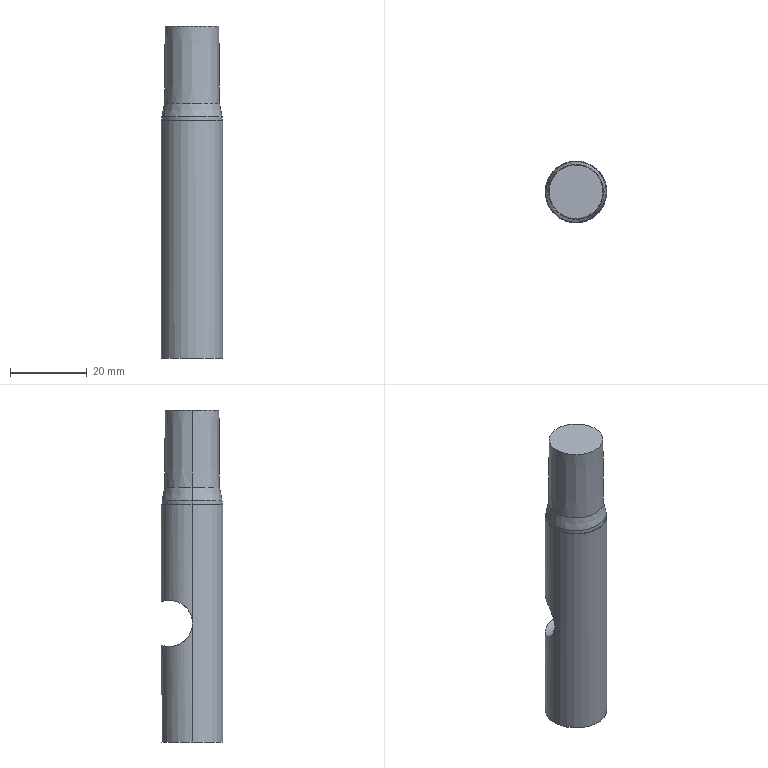Part | Creo | 1 solid | 13 faces | box 16.002 x 16 x 86.407 mm | volume 15399 mm3 | cylinder 6 | cone 4 | plane 3 | commonest cylinder face diameters 16 x3 15.678 x2 12 x1
STEP:
#1=CARTESIAN_POINT('',(0.,0.,0.));
#2=DIRECTION('',(0.,0.,1.));
#3=DIRECTION('',(1.,0.,0.));
#4=AXIS2_PLACEMENT_3D('',#1,#2,#3);
#5=CARTESIAN_POINT('',(104.477,27.678,-128.581));
#6=VERTEX_POINT('',#5);
#7=CARTESIAN_POINT('',(107.088,21.765,-123.596));
#8=VERTEX_POINT('',#7);
#9=CARTESIAN_POINT('',(104.477,27.678,-128.581));
#10=CARTESIAN_POINT('',(104.749,27.431,-128.581));
#11=CARTESIAN_POINT('',(105.24,26.915,-128.55));
#12=CARTESIAN_POINT('',(105.829,26.11,-128.393));
#13=CARTESIAN_POINT('',(106.284,25.299,-128.112));
#14=CARTESIAN_POINT('',(106.617,24.511,-127.704));
#15=CARTESIAN_POINT('',(106.849,23.756,-127.155));
#16=CARTESIAN_POINT('',(106.993,23.055,-126.45));
#17=CARTESIAN_POINT('',(107.064,22.455,-125.596));
#18=CARTESIAN_POINT('',(107.087,22.006,-124.63));
#19=CARTESIAN_POINT('',(107.088,21.826,-123.949));
#20=CARTESIAN_POINT('',(107.088,21.765,-123.596));
#21=B_SPLINE_CURVE_WITH_KNOTS('',3,(#9,#10,#11,#12,#13,#14,#15,#16,#17,#18,#19,#20),.UNSPECIFIED.,.F.,.F.,(4,1,1,1,1,1,1,1,1,4),(0.,0.1111,0.2222,0.3333,0.4444,0.5556,0.6667,0.7778,0.8889,1.),.UNSPECIFIED.);
#22=EDGE_CURVE('',#6,#8,#21,.T.);
#23=ORIENTED_EDGE('',*,*,#22,.T.);
#24=CARTESIAN_POINT('',(107.088,21.765,-121.572));
#25=VERTEX_POINT('',#24);
#26=CARTESIAN_POINT('',(107.088,21.765,-123.596));
#27=CARTESIAN_POINT('',(107.088,21.707,-123.258));
#28=CARTESIAN_POINT('',(107.087,21.65,-122.584));
#29=CARTESIAN_POINT('',(107.088,21.707,-121.909));
#30=CARTESIAN_POINT('',(107.088,21.765,-121.572));
#31=B_SPLINE_CURVE_WITH_KNOTS('',3,(#26,#27,#28,#29,#30),.UNSPECIFIED.,.F.,.F.,(4,1,4),(0.,0.5,1.),.UNSPECIFIED.);
#32=EDGE_CURVE('',#8,#25,#31,.T.);
#33=ORIENTED_EDGE('',*,*,#32,.T.);
#34=CARTESIAN_POINT('',(104.477,27.678,-116.581));
#35=VERTEX_POINT('',#34);
#36=CARTESIAN_POINT('',(107.088,21.765,-121.572));
#37=CARTESIAN_POINT('',(107.088,21.801,-121.361));
#38=CARTESIAN_POINT('',(107.087,21.894,-120.947));
#39=CARTESIAN_POINT('',(107.083,22.087,-120.374));
#40=CARTESIAN_POINT('',(107.067,22.369,-119.762));
#41=CARTESIAN_POINT('',(107.038,22.685,-119.235));
#42=CARTESIAN_POINT('',(106.982,23.089,-118.697));
#43=CARTESIAN_POINT('',(106.899,23.513,-118.25));
#44=CARTESIAN_POINT('',(106.79,23.947,-117.871));
#45=CARTESIAN_POINT('',(106.648,24.399,-117.547));
#46=CARTESIAN_POINT('',(106.469,24.864,-117.273));
#47=CARTESIAN_POINT('',(106.256,25.332,-117.051));
#48=CARTESIAN_POINT('',(105.99,25.823,-116.868));
#49=CARTESIAN_POINT('',(105.712,26.262,-116.745));
#50=CARTESIAN_POINT('',(105.379,26.72,-116.652));
#51=CARTESIAN_POINT('',(104.979,27.192,-116.595));
#52=CARTESIAN_POINT('',(104.654,27.517,-116.581));
#53=CARTESIAN_POINT('',(104.477,27.678,-116.581));
#54=B_SPLINE_CURVE_WITH_KNOTS('',3,(#36,#37,#38,#39,#40,#41,#42,#43,#44,#45,#46,#47,#48,#49,#50,#51,#52,#53),.UNSPECIFIED.,.F.,.F.,(4,1,1,1,1,1,1,1,1,1,1,1,1,1,1,4),(0.,0.06667,0.1333,0.2,0.2667,0.3333,0.4,0.4667,0.5333,0.6,0.6667,0.7333,0.8,0.8667,0.9333,1.),.UNSPECIFIED.);
#55=EDGE_CURVE('',#25,#35,#54,.T.);
#56=ORIENTED_EDGE('',*,*,#55,.T.);
#57=CARTESIAN_POINT('',(93.699,27.678,-116.581));
#58=VERTEX_POINT('',#57);
#59=CARTESIAN_POINT('',(104.158,27.97,-116.581));
#60=CARTESIAN_POINT('',(103.468,28.503,-116.623));
#61=CARTESIAN_POINT('',(102.306,29.13,-116.751));
#62=CARTESIAN_POINT('',(101.047,29.561,-116.881));
#63=CARTESIAN_POINT('',(99.717,29.78,-116.96));
#64=CARTESIAN_POINT('',(98.353,29.771,-116.957));
#65=CARTESIAN_POINT('',(97.016,29.532,-116.871));
#66=CARTESIAN_POINT('',(95.765,29.082,-116.739));
#67=CARTESIAN_POINT('',(94.636,28.453,-116.617));
#68=CARTESIAN_POINT('',(93.993,27.947,-116.581));
#69=CARTESIAN_POINT('',(93.699,27.678,-116.581));
#70=B_SPLINE_CURVE_WITH_KNOTS('',3,(#34,#59,#60,#61,#62,#63,#64,#65,#66,#67,#68,#69),.UNSPECIFIED.,.F.,.F.,(4,1,1,1,1,1,1,1,1,4),(0.,0.1111,0.2222,0.3333,0.4444,0.5556,0.6667,0.7778,0.8889,1.),.UNSPECIFIED.);
#71=EDGE_CURVE('',#35,#58,#70,.T.);
#72=ORIENTED_EDGE('',*,*,#71,.T.);
#73=CARTESIAN_POINT('',(91.087,21.766,-121.566));
#74=VERTEX_POINT('',#73);
#75=CARTESIAN_POINT('',(93.381,27.388,-116.581));
#76=CARTESIAN_POINT('',(92.819,26.782,-116.624));
#77=CARTESIAN_POINT('',(92.181,25.85,-116.839));
#78=CARTESIAN_POINT('',(91.72,24.934,-117.214));
#79=CARTESIAN_POINT('',(91.407,24.06,-117.757));
#80=CARTESIAN_POINT('',(91.218,23.266,-118.468));
#81=CARTESIAN_POINT('',(91.122,22.58,-119.351));
#82=CARTESIAN_POINT('',(91.09,22.053,-120.385));
#83=CARTESIAN_POINT('',(91.087,21.836,-121.157));
#84=CARTESIAN_POINT('',(91.087,21.766,-121.566));
#85=B_SPLINE_CURVE_WITH_KNOTS('',3,(#57,#75,#76,#77,#78,#79,#80,#81,#82,#83,#84),.UNSPECIFIED.,.F.,.F.,(4,1,1,1,1,1,1,1,4),(0.,0.125,0.25,0.375,0.5,0.625,0.75,0.875,1.),.UNSPECIFIED.);
#86=EDGE_CURVE('',#58,#74,#85,.T.);
#87=ORIENTED_EDGE('',*,*,#86,.T.);
#88=CARTESIAN_POINT('',(91.086,21.766,-123.595));
#89=VERTEX_POINT('',#88);
#90=CARTESIAN_POINT('',(91.087,21.766,-121.566));
#91=CARTESIAN_POINT('',(91.087,21.727,-121.79));
#92=CARTESIAN_POINT('',(91.089,21.675,-122.238));
#93=CARTESIAN_POINT('',(91.089,21.675,-122.921));
#94=CARTESIAN_POINT('',(91.086,21.727,-123.37));
#95=CARTESIAN_POINT('',(91.086,21.766,-123.595));
#96=B_SPLINE_CURVE_WITH_KNOTS('',3,(#90,#91,#92,#93,#94,#95),.UNSPECIFIED.,.F.,.F.,(4,1,1,4),(0.,0.3333,0.6667,1.),.UNSPECIFIED.);
#97=EDGE_CURVE('',#74,#89,#96,.T.);
#98=ORIENTED_EDGE('',*,*,#97,.T.);
#99=CARTESIAN_POINT('',(91.086,21.766,-123.595));
#100=CARTESIAN_POINT('',(91.086,21.837,-124.013));
#101=CARTESIAN_POINT('',(91.09,22.06,-124.799));
#102=CARTESIAN_POINT('',(91.123,22.603,-125.85));
#103=CARTESIAN_POINT('',(91.225,23.309,-126.743));
#104=CARTESIAN_POINT('',(91.427,24.128,-127.456));
#105=CARTESIAN_POINT('',(91.756,25.017,-127.991));
#106=CARTESIAN_POINT('',(92.243,25.955,-128.356));
#107=CARTESIAN_POINT('',(92.919,26.907,-128.556));
#108=CARTESIAN_POINT('',(93.806,27.823,-128.601));
#109=CARTESIAN_POINT('',(94.912,28.639,-128.519));
#110=CARTESIAN_POINT('',(96.214,29.28,-128.372));
#111=CARTESIAN_POINT('',(97.645,29.682,-128.239));
#112=CARTESIAN_POINT('',(99.145,29.812,-128.189));
#113=CARTESIAN_POINT('',(100.628,29.663,-128.246));
#114=CARTESIAN_POINT('',(102.045,29.248,-128.381));
#115=CARTESIAN_POINT('',(103.356,28.584,-128.529));
#116=CARTESIAN_POINT('',(104.124,28.,-128.581));
#117=B_SPLINE_CURVE_WITH_KNOTS('',3,(#99,#100,#101,#102,#103,#104,#105,#106,#107,#108,#109,#110,#111,#112,#113,#114,#115,#116,#5),.UNSPECIFIED.,.F.,.F.,(4,1,1,1,1,1,1,1,1,1,1,1,1,1,1,1,4),(0.,0.0625,0.125,0.1875,0.25,0.3125,0.375,0.4375,0.5,0.5625,0.625,0.6875,0.75,0.8125,0.875,0.9375,1.),.UNSPECIFIED.);
#118=EDGE_CURVE('',#89,#6,#117,.T.);
#119=ORIENTED_EDGE('',*,*,#118,.T.);
#120=EDGE_LOOP('',(#23,#33,#56,#72,#87,#98,#119));
#121=FACE_OUTER_BOUND('',#120,.F.);
#122=CARTESIAN_POINT('',(389.101,27.678,-122.581));
#123=DIRECTION('',(-1.,0.,0.));
#124=DIRECTION('',(0.,0.,1.));
#125=AXIS2_PLACEMENT_3D('',#122,#123,#124);
#126=CYLINDRICAL_SURFACE('',#125,6.);
#127=ADVANCED_FACE('',(#121),#126,.F.);
#128=ORIENTED_EDGE('',*,*,#86,.F.);
#129=ORIENTED_EDGE('',*,*,#71,.F.);
#130=ORIENTED_EDGE('',*,*,#55,.F.);
#131=CARTESIAN_POINT('',(107.088,21.766,-91.655));
#132=VERTEX_POINT('',#131);
#133=CARTESIAN_POINT('',(107.088,21.766,-91.655));
#134=DIRECTION('',(0.000003841,-0.00004371,-1.));
#135=VECTOR('',#134,29.916);
#136=LINE('',#133,#135);
#137=EDGE_CURVE('',#132,#25,#136,.T.);
#138=ORIENTED_EDGE('',*,*,#137,.F.);
#139=CARTESIAN_POINT('',(91.088,21.776,-91.634));
#140=VERTEX_POINT('',#139);
#141=CARTESIAN_POINT('',(91.089,22.719,-91.634));
#142=CARTESIAN_POINT('',(91.433,24.755,-91.635));
#143=CARTESIAN_POINT('',(92.963,27.121,-91.637));
#144=CARTESIAN_POINT('',(94.691,28.516,-91.639));
#145=CARTESIAN_POINT('',(96.14,29.26,-91.641));
#146=CARTESIAN_POINT('',(97.393,29.613,-91.643));
#147=CARTESIAN_POINT('',(98.379,29.746,-91.644));
#148=CARTESIAN_POINT('',(99.093,29.776,-91.645));
#149=CARTESIAN_POINT('',(99.808,29.745,-91.646));
#150=CARTESIAN_POINT('',(100.793,29.61,-91.647));
#151=CARTESIAN_POINT('',(102.045,29.256,-91.649));
#152=CARTESIAN_POINT('',(103.494,28.51,-91.651));
#153=CARTESIAN_POINT('',(105.22,27.113,-91.653));
#154=CARTESIAN_POINT('',(106.747,24.745,-91.655));
#155=CARTESIAN_POINT('',(107.088,22.708,-91.655));
#156=B_SPLINE_CURVE_WITH_KNOTS('',3,(#139,#141,#142,#143,#144,#145,#146,#147,#148,#149,#150,#151,#152,#153,#154,#155,#131),.UNSPECIFIED.,.F.,.F.,(4,1,1,1,1,1,1,1,1,1,1,1,1,1,4),(0.,0.125,0.25,0.3125,0.375,0.4375,0.4688,0.5,0.5312,0.5625,0.625,0.6875,0.75,0.875,1.),.UNSPECIFIED.);
#157=EDGE_CURVE('',#140,#132,#156,.T.);
#158=ORIENTED_EDGE('',*,*,#157,.F.);
#159=CARTESIAN_POINT('',(91.088,21.766,-91.634));
#160=VERTEX_POINT('',#159);
#161=CARTESIAN_POINT('',(91.088,21.769,-91.634));
#162=CARTESIAN_POINT('',(91.088,21.773,-91.634));
#163=CARTESIAN_POINT('',(91.088,21.776,-91.634));
#164=B_SPLINE_CURVE_WITH_KNOTS('',3,(#159,#161,#162,#163),.UNSPECIFIED.,.F.,.F.,(4,4),(0.,1.),.UNSPECIFIED.);
#165=EDGE_CURVE('',#160,#140,#164,.T.);
#166=ORIENTED_EDGE('',*,*,#165,.F.);
#167=CARTESIAN_POINT('',(91.088,21.766,-91.634));
#168=DIRECTION('',(-0.00004459,-0.0000106,-1.));
#169=VECTOR('',#168,29.932);
#170=LINE('',#167,#169);
#171=EDGE_CURVE('',#160,#74,#170,.T.);
#172=ORIENTED_EDGE('',*,*,#171,.T.);
#173=EDGE_LOOP('',(#128,#129,#130,#138,#158,#166,#172));
#174=FACE_OUTER_BOUND('',#173,.F.);
#175=CARTESIAN_POINT('',(99.088,21.766,508.193));
#176=DIRECTION('',(0.,0.,-1.));
#177=DIRECTION('',(-1.,0.,0.));
#178=AXIS2_PLACEMENT_3D('',#175,#176,#177);
#179=CYLINDRICAL_SURFACE('',#178,8.);
#180=ADVANCED_FACE('',(#174),#179,.T.);
#181=ORIENTED_EDGE('',*,*,#118,.F.);
#182=CARTESIAN_POINT('',(91.088,21.766,-153.441));
#183=VERTEX_POINT('',#182);
#184=CARTESIAN_POINT('',(91.086,21.766,-123.595));
#185=DIRECTION('',(0.00005964,0.00001266,-1.));
#186=VECTOR('',#185,29.847);
#187=LINE('',#184,#186);
#188=EDGE_CURVE('',#89,#183,#187,.T.);
#189=ORIENTED_EDGE('',*,*,#188,.T.);
#190=CARTESIAN_POINT('',(107.088,21.766,-153.441));
#191=VERTEX_POINT('',#190);
#192=CARTESIAN_POINT('',(99.088,21.766,-153.441));
#193=DIRECTION('',(0.,0.,-1.));
#194=DIRECTION('',(-1.,0.,0.));
#195=AXIS2_PLACEMENT_3D('',#192,#193,#194);
#196=CIRCLE('',#195,8.);
#197=EDGE_CURVE('',#183,#191,#196,.T.);
#198=ORIENTED_EDGE('',*,*,#197,.T.);
#199=CARTESIAN_POINT('',(107.088,21.765,-123.596));
#200=DIRECTION('',(-0.000003617,0.00002334,-1.));
#201=VECTOR('',#200,29.846);
#202=LINE('',#199,#201);
#203=EDGE_CURVE('',#8,#191,#202,.T.);
#204=ORIENTED_EDGE('',*,*,#203,.F.);
#205=ORIENTED_EDGE('',*,*,#22,.F.);
#206=EDGE_LOOP('',(#181,#189,#198,#204,#205));
#207=FACE_OUTER_BOUND('',#206,.F.);
#208=CARTESIAN_POINT('',(99.088,21.766,508.193));
#209=DIRECTION('',(0.,0.,-1.));
#210=DIRECTION('',(-1.,0.,0.));
#211=AXIS2_PLACEMENT_3D('',#208,#209,#210);
#212=CYLINDRICAL_SURFACE('',#211,8.);
#213=ADVANCED_FACE('',(#207),#212,.T.);
#214=ORIENTED_EDGE('',*,*,#97,.F.);
#215=ORIENTED_EDGE('',*,*,#171,.F.);
#216=CARTESIAN_POINT('',(107.088,21.756,-91.655));
#217=VERTEX_POINT('',#216);
#218=CARTESIAN_POINT('',(107.087,21.26,-91.655));
#219=CARTESIAN_POINT('',(106.996,20.286,-91.655));
#220=CARTESIAN_POINT('',(106.59,18.856,-91.655));
#221=CARTESIAN_POINT('',(105.925,17.525,-91.654));
#222=CARTESIAN_POINT('',(105.039,16.351,-91.653));
#223=CARTESIAN_POINT('',(103.938,15.345,-91.651));
#224=CARTESIAN_POINT('',(102.67,14.561,-91.65));
#225=CARTESIAN_POINT('',(101.281,14.025,-91.648));
#226=CARTESIAN_POINT('',(99.821,13.754,-91.646));
#227=CARTESIAN_POINT('',(98.339,13.755,-91.644));
#228=CARTESIAN_POINT('',(96.883,14.029,-91.642));
#229=CARTESIAN_POINT('',(95.502,14.564,-91.64));
#230=CARTESIAN_POINT('',(94.241,15.344,-91.639));
#231=CARTESIAN_POINT('',(93.143,16.345,-91.637));
#232=CARTESIAN_POINT('',(92.256,17.518,-91.636));
#233=CARTESIAN_POINT('',(91.588,18.851,-91.635));
#234=CARTESIAN_POINT('',(91.18,20.288,-91.635));
#235=CARTESIAN_POINT('',(91.088,21.267,-91.634));
#236=CARTESIAN_POINT('',(91.088,21.766,-91.634));
#237=B_SPLINE_CURVE_WITH_KNOTS('',3,(#216,#218,#219,#220,#221,#222,#223,#224,#225,#226,#227,#228,#229,#230,#231,#232,#233,#234,#235,#236),.UNSPECIFIED.,.F.,.F.,(4,1,1,1,1,1,1,1,1,1,1,1,1,1,1,1,1,4),(0.,0.05882,0.1176,0.1765,0.2353,0.2941,0.3529,0.4118,0.4706,0.5294,0.5882,0.6471,0.7059,0.7647,0.8235,0.8824,0.9412,1.),.UNSPECIFIED.);
#238=EDGE_CURVE('',#217,#160,#237,.T.);
#239=ORIENTED_EDGE('',*,*,#238,.F.);
#240=CARTESIAN_POINT('',(107.088,21.766,-91.655));
#241=CARTESIAN_POINT('',(107.088,21.763,-91.655));
#242=CARTESIAN_POINT('',(107.088,21.759,-91.655));
#243=CARTESIAN_POINT('',(107.088,21.756,-91.655));
#244=B_SPLINE_CURVE_WITH_KNOTS('',3,(#240,#241,#242,#243),.UNSPECIFIED.,.F.,.F.,(4,4),(0.,1.),.UNSPECIFIED.);
#245=EDGE_CURVE('',#132,#217,#244,.T.);
#246=ORIENTED_EDGE('',*,*,#245,.F.);
#247=ORIENTED_EDGE('',*,*,#137,.T.);
#248=ORIENTED_EDGE('',*,*,#32,.F.);
#249=ORIENTED_EDGE('',*,*,#203,.T.);
#250=CARTESIAN_POINT('',(99.088,21.766,-153.441));
#251=DIRECTION('',(0.,0.,-1.));
#252=DIRECTION('',(1.,0.,0.));
#253=AXIS2_PLACEMENT_3D('',#250,#251,#252);
#254=CIRCLE('',#253,8.);
#255=EDGE_CURVE('',#191,#183,#254,.T.);
#256=ORIENTED_EDGE('',*,*,#255,.T.);
#257=ORIENTED_EDGE('',*,*,#188,.F.);
#258=EDGE_LOOP('',(#214,#215,#239,#246,#247,#248,#249,#256,#257));
#259=FACE_OUTER_BOUND('',#258,.F.);
#260=CARTESIAN_POINT('',(99.088,21.766,508.193));
#261=DIRECTION('',(0.,0.,-1.));
#262=DIRECTION('',(-1.,0.,0.));
#263=AXIS2_PLACEMENT_3D('',#260,#261,#262);
#264=CYLINDRICAL_SURFACE('',#263,8.);
#265=ADVANCED_FACE('',(#259),#264,.T.);
#266=ORIENTED_EDGE('',*,*,#238,.T.);
#267=ORIENTED_EDGE('',*,*,#165,.T.);
#268=ORIENTED_EDGE('',*,*,#157,.T.);
#269=ORIENTED_EDGE('',*,*,#245,.T.);
#270=EDGE_LOOP('',(#266,#267,#268,#269));
#271=FACE_OUTER_BOUND('',#270,.F.);
#272=CARTESIAN_POINT('',(106.927,21.756,-91.655));
#273=VERTEX_POINT('',#272);
#274=CARTESIAN_POINT('',(106.927,21.766,-91.655));
#275=VERTEX_POINT('',#274);
#276=CARTESIAN_POINT('',(106.927,21.759,-91.655));
#277=CARTESIAN_POINT('',(106.927,21.763,-91.655));
#278=CARTESIAN_POINT('',(106.927,21.766,-91.655));
#279=B_SPLINE_CURVE_WITH_KNOTS('',3,(#272,#276,#277,#278),.UNSPECIFIED.,.F.,.F.,(4,4),(0.,1.),.UNSPECIFIED.);
#280=EDGE_CURVE('',#273,#275,#279,.T.);
#281=ORIENTED_EDGE('',*,*,#280,.T.);
#282=CARTESIAN_POINT('',(91.249,21.776,-91.635));
#283=VERTEX_POINT('',#282);
#284=CARTESIAN_POINT('',(106.927,22.252,-91.655));
#285=CARTESIAN_POINT('',(106.838,23.206,-91.655));
#286=CARTESIAN_POINT('',(106.442,24.608,-91.655));
#287=CARTESIAN_POINT('',(105.792,25.913,-91.654));
#288=CARTESIAN_POINT('',(104.926,27.064,-91.653));
#289=CARTESIAN_POINT('',(103.848,28.051,-91.651));
#290=CARTESIAN_POINT('',(102.607,28.821,-91.65));
#291=CARTESIAN_POINT('',(101.247,29.348,-91.648));
#292=CARTESIAN_POINT('',(99.817,29.616,-91.646));
#293=CARTESIAN_POINT('',(98.364,29.616,-91.644));
#294=CARTESIAN_POINT('',(96.938,29.35,-91.642));
#295=CARTESIAN_POINT('',(95.584,28.828,-91.64));
#296=CARTESIAN_POINT('',(94.347,28.065,-91.639));
#297=CARTESIAN_POINT('',(93.27,27.085,-91.637));
#298=CARTESIAN_POINT('',(92.399,25.937,-91.636));
#299=CARTESIAN_POINT('',(91.742,24.631,-91.635));
#300=CARTESIAN_POINT('',(91.341,23.224,-91.635));
#301=CARTESIAN_POINT('',(91.25,22.265,-91.635));
#302=CARTESIAN_POINT('',(91.249,21.776,-91.635));
#303=B_SPLINE_CURVE_WITH_KNOTS('',3,(#274,#284,#285,#286,#287,#288,#289,#290,#291,#292,#293,#294,#295,#296,#297,#298,#299,#300,#301,#302),.UNSPECIFIED.,.F.,.F.,(4,1,1,1,1,1,1,1,1,1,1,1,1,1,1,1,1,4),(0.,0.05882,0.1176,0.1765,0.2353,0.2941,0.3529,0.4118,0.4706,0.5294,0.5882,0.6471,0.7059,0.7647,0.8235,0.8824,0.9412,1.),.UNSPECIFIED.);
#304=EDGE_CURVE('',#275,#283,#303,.T.);
#305=ORIENTED_EDGE('',*,*,#304,.T.);
#306=CARTESIAN_POINT('',(91.249,21.766,-91.635));
#307=VERTEX_POINT('',#306);
#308=CARTESIAN_POINT('',(91.249,21.773,-91.635));
#309=CARTESIAN_POINT('',(91.249,21.769,-91.635));
#310=B_SPLINE_CURVE_WITH_KNOTS('',3,(#282,#308,#309,#306),.UNSPECIFIED.,.F.,.F.,(4,4),(0.,1.),.UNSPECIFIED.);
#311=EDGE_CURVE('',#283,#307,#310,.T.);
#312=ORIENTED_EDGE('',*,*,#311,.T.);
#313=CARTESIAN_POINT('',(91.249,21.766,-91.635));
#314=CARTESIAN_POINT('',(91.249,20.842,-91.635));
#315=CARTESIAN_POINT('',(91.584,18.846,-91.635));
#316=CARTESIAN_POINT('',(93.079,16.526,-91.637));
#317=CARTESIAN_POINT('',(94.771,15.157,-91.639));
#318=CARTESIAN_POINT('',(96.19,14.426,-91.641));
#319=CARTESIAN_POINT('',(97.417,14.079,-91.643));
#320=CARTESIAN_POINT('',(98.383,13.948,-91.644));
#321=CARTESIAN_POINT('',(99.083,13.917,-91.645));
#322=CARTESIAN_POINT('',(99.783,13.947,-91.646));
#323=CARTESIAN_POINT('',(100.749,14.077,-91.647));
#324=CARTESIAN_POINT('',(101.977,14.423,-91.649));
#325=CARTESIAN_POINT('',(103.397,15.152,-91.651));
#326=CARTESIAN_POINT('',(105.09,16.519,-91.653));
#327=CARTESIAN_POINT('',(106.589,18.837,-91.655));
#328=CARTESIAN_POINT('',(106.926,20.832,-91.655));
#329=CARTESIAN_POINT('',(106.927,21.756,-91.655));
#330=B_SPLINE_CURVE_WITH_KNOTS('',3,(#313,#314,#315,#316,#317,#318,#319,#320,#321,#322,#323,#324,#325,#326,#327,#328,#329),.UNSPECIFIED.,.F.,.F.,(4,1,1,1,1,1,1,1,1,1,1,1,1,1,4),(0.,0.125,0.25,0.3125,0.375,0.4375,0.4688,0.5,0.5312,0.5625,0.625,0.6875,0.75,0.875,1.),.UNSPECIFIED.);
#331=EDGE_CURVE('',#307,#273,#330,.T.);
#332=ORIENTED_EDGE('',*,*,#331,.T.);
#333=EDGE_LOOP('',(#281,#305,#312,#332));
#334=FACE_BOUND('',#333,.F.);
#335=CARTESIAN_POINT('',(248.993,54.022,-91.842));
#336=DIRECTION('',(-0.001312,0.000001665,-1.));
#337=DIRECTION('',(-1.,0.,0.001312));
#338=AXIS2_PLACEMENT_3D('',#335,#336,#337);
#339=PLANE('',#338);
#340=ADVANCED_FACE('',(#271,#334),#339,.F.);
#341=CARTESIAN_POINT('',(91.248,21.766,-90.64));
#342=VERTEX_POINT('',#341);
#343=CARTESIAN_POINT('',(106.927,21.766,-90.64));
#344=VERTEX_POINT('',#343);
#345=CARTESIAN_POINT('',(99.087,21.766,-90.64));
#346=DIRECTION('',(0.00002709,0.,1.));
#347=DIRECTION('',(-1.,0.,0.00002709));
#348=AXIS2_PLACEMENT_3D('',#345,#346,#347);
#349=CIRCLE('',#348,7.841);
#350=EDGE_CURVE('',#342,#344,#349,.T.);
#351=ORIENTED_EDGE('',*,*,#350,.T.);
#352=CARTESIAN_POINT('',(106.927,21.766,-91.655));
#353=DIRECTION('',(0.0003926,0.000000008,1.));
#354=VECTOR('',#353,1.015);
#355=LINE('',#352,#354);
#356=EDGE_CURVE('',#275,#344,#355,.T.);
#357=ORIENTED_EDGE('',*,*,#356,.F.);
#358=ORIENTED_EDGE('',*,*,#280,.F.);
#359=ORIENTED_EDGE('',*,*,#331,.F.);
#360=CARTESIAN_POINT('',(91.249,21.766,-91.635));
#361=DIRECTION('',(-0.001462,0.,1.));
#362=VECTOR('',#361,0.995);
#363=LINE('',#360,#362);
#364=EDGE_CURVE('',#307,#342,#363,.T.);
#365=ORIENTED_EDGE('',*,*,#364,.T.);
#366=EDGE_LOOP('',(#351,#357,#358,#359,#365));
#367=FACE_OUTER_BOUND('',#366,.F.);
#368=CARTESIAN_POINT('',(99.088,21.766,-91.645));
#369=DIRECTION('',(0.,0.,1.));
#370=DIRECTION('',(1.,0.,0.));
#371=AXIS2_PLACEMENT_3D('',#368,#369,#370);
#372=CYLINDRICAL_SURFACE('',#371,7.839);
#373=ADVANCED_FACE('',(#367),#372,.T.);
#374=CARTESIAN_POINT('',(91.951,21.766,-87.122));
#375=VERTEX_POINT('',#374);
#376=CARTESIAN_POINT('',(106.224,21.766,-87.122));
#377=VERTEX_POINT('',#376);
#378=CARTESIAN_POINT('',(99.088,21.766,-87.122));
#379=DIRECTION('',(0.,0.,1.));
#380=DIRECTION('',(-1.,0.,0.));
#381=AXIS2_PLACEMENT_3D('',#378,#379,#380);
#382=CIRCLE('',#381,7.136);
#383=EDGE_CURVE('',#375,#377,#382,.T.);
#384=ORIENTED_EDGE('',*,*,#383,.T.);
#385=CARTESIAN_POINT('',(106.224,21.766,-87.122));
#386=DIRECTION('',(0.1961,0.,-0.9806));
#387=VECTOR('',#386,3.587);
#388=LINE('',#385,#387);
#389=EDGE_CURVE('',#377,#344,#388,.T.);
#390=ORIENTED_EDGE('',*,*,#389,.T.);
#391=ORIENTED_EDGE('',*,*,#350,.F.);
#392=CARTESIAN_POINT('',(91.951,21.766,-87.122));
#393=DIRECTION('',(-0.1962,0.,-0.9806));
#394=VECTOR('',#393,3.587);
#395=LINE('',#392,#394);
#396=EDGE_CURVE('',#375,#342,#395,.T.);
#397=ORIENTED_EDGE('',*,*,#396,.F.);
#398=EDGE_LOOP('',(#384,#390,#391,#397));
#399=FACE_OUTER_BOUND('',#398,.F.);
#400=CARTESIAN_POINT('',(99.087,21.766,-88.881));
#401=DIRECTION('',(-0.00002709,0.,-1.));
#402=DIRECTION('',(1.,0.,-0.00002709));
#403=AXIS2_PLACEMENT_3D('',#400,#401,#402);
#404=CONICAL_SURFACE('',#403,7.489,11.313);
#405=ADVANCED_FACE('',(#399),#404,.T.);
#406=ORIENTED_EDGE('',*,*,#383,.F.);
#407=CARTESIAN_POINT('',(92.092,21.766,-67.098));
#408=VERTEX_POINT('',#407);
#409=CARTESIAN_POINT('',(92.092,21.766,-67.098));
#410=DIRECTION('',(-0.007048,0.,-1.));
#411=VECTOR('',#410,20.025);
#412=LINE('',#409,#411);
#413=EDGE_CURVE('',#408,#375,#412,.T.);
#414=ORIENTED_EDGE('',*,*,#413,.F.);
#415=CARTESIAN_POINT('',(106.084,21.766,-67.116));
#416=VERTEX_POINT('',#415);
#417=CARTESIAN_POINT('',(92.092,21.766,-67.098));
#418=CARTESIAN_POINT('',(92.092,20.941,-67.089));
#419=CARTESIAN_POINT('',(92.391,19.16,-67.071));
#420=CARTESIAN_POINT('',(93.727,17.089,-67.052));
#421=CARTESIAN_POINT('',(95.238,15.867,-67.041));
#422=CARTESIAN_POINT('',(96.504,15.215,-67.036));
#423=CARTESIAN_POINT('',(97.825,14.844,-67.034));
#424=CARTESIAN_POINT('',(99.088,14.734,-67.035));
#425=CARTESIAN_POINT('',(100.351,14.844,-67.037));
#426=CARTESIAN_POINT('',(101.672,15.215,-67.043));
#427=CARTESIAN_POINT('',(102.938,15.867,-67.051));
#428=CARTESIAN_POINT('',(104.449,17.089,-67.066));
#429=CARTESIAN_POINT('',(105.785,19.16,-67.089));
#430=CARTESIAN_POINT('',(106.084,20.941,-67.108));
#431=CARTESIAN_POINT('',(106.084,21.766,-67.116));
#432=B_SPLINE_CURVE_WITH_KNOTS('',3,(#417,#418,#419,#420,#421,#422,#423,#424,#425,#426,#427,#428,#429,#430,#431),.UNSPECIFIED.,.F.,.F.,(4,1,1,1,1,1,1,1,1,1,1,1,4),(0.,0.125,0.25,0.3125,0.375,0.4375,0.5,0.5625,0.625,0.6875,0.75,0.875,1.),.UNSPECIFIED.);
#433=EDGE_CURVE('',#408,#416,#432,.T.);
#434=ORIENTED_EDGE('',*,*,#433,.T.);
#435=CARTESIAN_POINT('',(106.084,21.766,-67.116));
#436=DIRECTION('',(0.007,0.,-1.));
#437=VECTOR('',#436,20.007);
#438=LINE('',#435,#437);
#439=EDGE_CURVE('',#416,#377,#438,.T.);
#440=ORIENTED_EDGE('',*,*,#439,.T.);
#441=EDGE_LOOP('',(#406,#414,#434,#440));
#442=FACE_OUTER_BOUND('',#441,.F.);
#443=CARTESIAN_POINT('',(99.088,21.766,-77.078));
#444=DIRECTION('',(0.,0.,-1.));
#445=DIRECTION('',(1.,0.,0.));
#446=AXIS2_PLACEMENT_3D('',#443,#444,#445);
#447=CONICAL_SURFACE('',#446,7.065,0.4);
#448=ADVANCED_FACE('',(#442),#447,.T.);
#449=CARTESIAN_POINT('',(99.088,21.766,-87.122));
#450=DIRECTION('',(0.,0.,1.));
#451=DIRECTION('',(1.,0.,0.));
#452=AXIS2_PLACEMENT_3D('',#449,#450,#451);
#453=CIRCLE('',#452,7.136);
#454=EDGE_CURVE('',#377,#375,#453,.T.);
#455=ORIENTED_EDGE('',*,*,#454,.F.);
#456=ORIENTED_EDGE('',*,*,#439,.F.);
#457=CARTESIAN_POINT('',(99.968,28.707,-67.18));
#458=VERTEX_POINT('',#457);
#459=CARTESIAN_POINT('',(106.084,21.766,-67.116));
#460=CARTESIAN_POINT('',(106.084,22.28,-67.121));
#461=CARTESIAN_POINT('',(105.975,23.211,-67.131));
#462=CARTESIAN_POINT('',(105.473,24.824,-67.147));
#463=CARTESIAN_POINT('',(104.429,26.473,-67.162));
#464=CARTESIAN_POINT('',(102.925,27.716,-67.173));
#465=CARTESIAN_POINT('',(101.388,28.417,-67.178));
#466=CARTESIAN_POINT('',(100.477,28.642,-67.18));
#467=B_SPLINE_CURVE_WITH_KNOTS('',3,(#459,#460,#461,#462,#463,#464,#465,#466,#457),.UNSPECIFIED.,.F.,.F.,(4,1,1,1,1,1,4),(0.,0.125,0.25,0.5,0.75,0.875,1.),.UNSPECIFIED.);
#468=EDGE_CURVE('',#416,#458,#467,.T.);
#469=ORIENTED_EDGE('',*,*,#468,.T.);
#470=CARTESIAN_POINT('',(99.968,28.707,-67.18));
#471=CARTESIAN_POINT('',(99.311,28.79,-67.18));
#472=CARTESIAN_POINT('',(98.172,28.759,-67.178));
#473=CARTESIAN_POINT('',(96.257,28.286,-67.17));
#474=CARTESIAN_POINT('',(94.36,27.131,-67.156));
#475=CARTESIAN_POINT('',(92.976,25.394,-67.136));
#476=CARTESIAN_POINT('',(92.266,23.554,-67.117));
#477=CARTESIAN_POINT('',(92.092,22.427,-67.105));
#478=CARTESIAN_POINT('',(92.092,21.766,-67.098));
#479=B_SPLINE_CURVE_WITH_KNOTS('',3,(#470,#471,#472,#473,#474,#475,#476,#477,#478),.UNSPECIFIED.,.F.,.F.,(4,1,1,1,1,1,4),(0.,0.125,0.25,0.5,0.75,0.875,1.),.UNSPECIFIED.);
#480=EDGE_CURVE('',#458,#408,#479,.T.);
#481=ORIENTED_EDGE('',*,*,#480,.T.);
#482=ORIENTED_EDGE('',*,*,#413,.T.);
#483=EDGE_LOOP('',(#455,#456,#469,#481,#482));
#484=FACE_OUTER_BOUND('',#483,.F.);
#485=CARTESIAN_POINT('',(99.088,21.766,-77.11));
#486=DIRECTION('',(0.,0.,-1.));
#487=DIRECTION('',(1.,0.,0.));
#488=AXIS2_PLACEMENT_3D('',#485,#486,#487);
#489=CONICAL_SURFACE('',#488,7.066,0.4);
#490=ADVANCED_FACE('',(#484),#489,.T.);
#491=ORIENTED_EDGE('',*,*,#454,.T.);
#492=ORIENTED_EDGE('',*,*,#396,.T.);
#493=CARTESIAN_POINT('',(99.087,21.766,-90.64));
#494=DIRECTION('',(0.00002709,0.,1.));
#495=DIRECTION('',(1.,0.,-0.00002709));
#496=AXIS2_PLACEMENT_3D('',#493,#494,#495);
#497=CIRCLE('',#496,7.841);
#498=EDGE_CURVE('',#344,#342,#497,.T.);
#499=ORIENTED_EDGE('',*,*,#498,.F.);
#500=ORIENTED_EDGE('',*,*,#389,.F.);
#501=EDGE_LOOP('',(#491,#492,#499,#500));
#502=FACE_OUTER_BOUND('',#501,.F.);
#503=CARTESIAN_POINT('',(99.087,21.766,-88.881));
#504=DIRECTION('',(-0.00002709,0.,-1.));
#505=DIRECTION('',(1.,0.,-0.00002709));
#506=AXIS2_PLACEMENT_3D('',#503,#504,#505);
#507=CONICAL_SURFACE('',#506,7.489,11.313);
#508=ADVANCED_FACE('',(#502),#507,.T.);
#509=ORIENTED_EDGE('',*,*,#498,.T.);
#510=ORIENTED_EDGE('',*,*,#364,.F.);
#511=ORIENTED_EDGE('',*,*,#311,.F.);
#512=ORIENTED_EDGE('',*,*,#304,.F.);
#513=ORIENTED_EDGE('',*,*,#356,.T.);
#514=EDGE_LOOP('',(#509,#510,#511,#512,#513));
#515=FACE_OUTER_BOUND('',#514,.F.);
#516=CARTESIAN_POINT('',(99.088,21.766,-91.645));
#517=DIRECTION('',(0.,0.,1.));
#518=DIRECTION('',(1.,0.,0.));
#519=AXIS2_PLACEMENT_3D('',#516,#517,#518);
#520=CYLINDRICAL_SURFACE('',#519,7.839);
#521=ADVANCED_FACE('',(#515),#520,.T.);
#522=ORIENTED_EDGE('',*,*,#480,.F.);
#523=ORIENTED_EDGE('',*,*,#468,.F.);
#524=ORIENTED_EDGE('',*,*,#433,.F.);
#525=EDGE_LOOP('',(#522,#523,#524));
#526=FACE_OUTER_BOUND('',#525,.F.);
#527=CARTESIAN_POINT('',(69.971,34.571,-67.201));
#528=DIRECTION('',(-0.001305,-0.0103,-0.9999));
#529=DIRECTION('',(0.,0.9999,-0.0103));
#530=AXIS2_PLACEMENT_3D('',#527,#528,#529);
#531=PLANE('',#530);
#532=ADVANCED_FACE('',(#526),#531,.F.);
#533=ORIENTED_EDGE('',*,*,#197,.F.);
#534=ORIENTED_EDGE('',*,*,#255,.F.);
#535=EDGE_LOOP('',(#533,#534));
#536=FACE_OUTER_BOUND('',#535,.F.);
#537=CARTESIAN_POINT('',(5.725,319.968,-153.441));
#538=DIRECTION('',(0.,0.,-1.));
#539=DIRECTION('',(-1.,0.,0.));
#540=AXIS2_PLACEMENT_3D('',#537,#538,#539);
#541=PLANE('',#540);
#542=ADVANCED_FACE('',(#536),#541,.T.);
#543=CLOSED_SHELL('',(#127,#180,#213,#265,#340,#373,#405,#448,#490,#508,#521,#532,#542));
#544=MANIFOLD_SOLID_BREP('',#543);
#545=(LENGTH_UNIT()NAMED_UNIT(*)SI_UNIT(.MILLI.,.METRE.));
#546=UNCERTAINTY_MEASURE_WITH_UNIT(LENGTH_MEASURE(0.008933),#545,'','');
#547=(NAMED_UNIT(*)PLANE_ANGLE_UNIT()SI_UNIT($,.RADIAN.));
#548=PLANE_ANGLE_MEASURE_WITH_UNIT(PLANE_ANGLE_MEASURE(0.01745),#547);
#549=(CONVERSION_BASED_UNIT('DEGREE',#548)NAMED_UNIT(*)PLANE_ANGLE_UNIT());
#550=(NAMED_UNIT(*)SI_UNIT($,.STERADIAN.)SOLID_ANGLE_UNIT());
#551=(GEOMETRIC_REPRESENTATION_CONTEXT(3)GLOBAL_UNCERTAINTY_ASSIGNED_CONTEXT((#546))GLOBAL_UNIT_ASSIGNED_CONTEXT((#545,#549,#550))REPRESENTATION_CONTEXT('',''));
#552=ADVANCED_BREP_SHAPE_REPRESENTATION('',(#4,#544),#551);